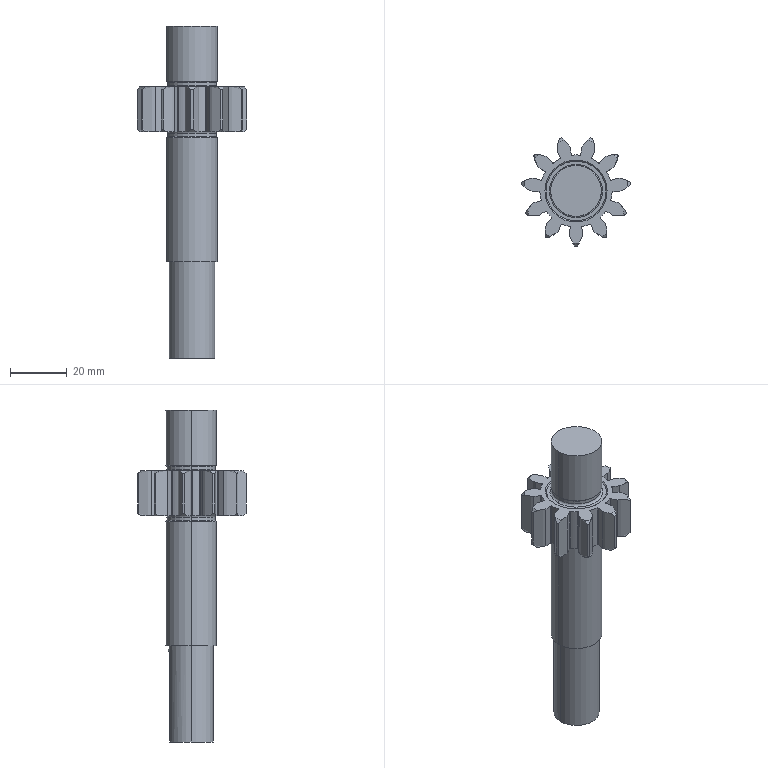Part | SolidWorks | features ICE 5, Fillet 3, CirPattern 2, Chamfer 1, Extrusion 1, RevCut 1 | 1 solid | 148 faces | box 38.703 x 38.313 x 117.5 mm | volume 35920 mm3 | cylinder 60 | plane 32 | cone 30 | spline 22 | torus 4 | commonest cylinder face diameters 0.6 x27 25.5 x11 39 x11 17.2 x4 18 x4 16 x2